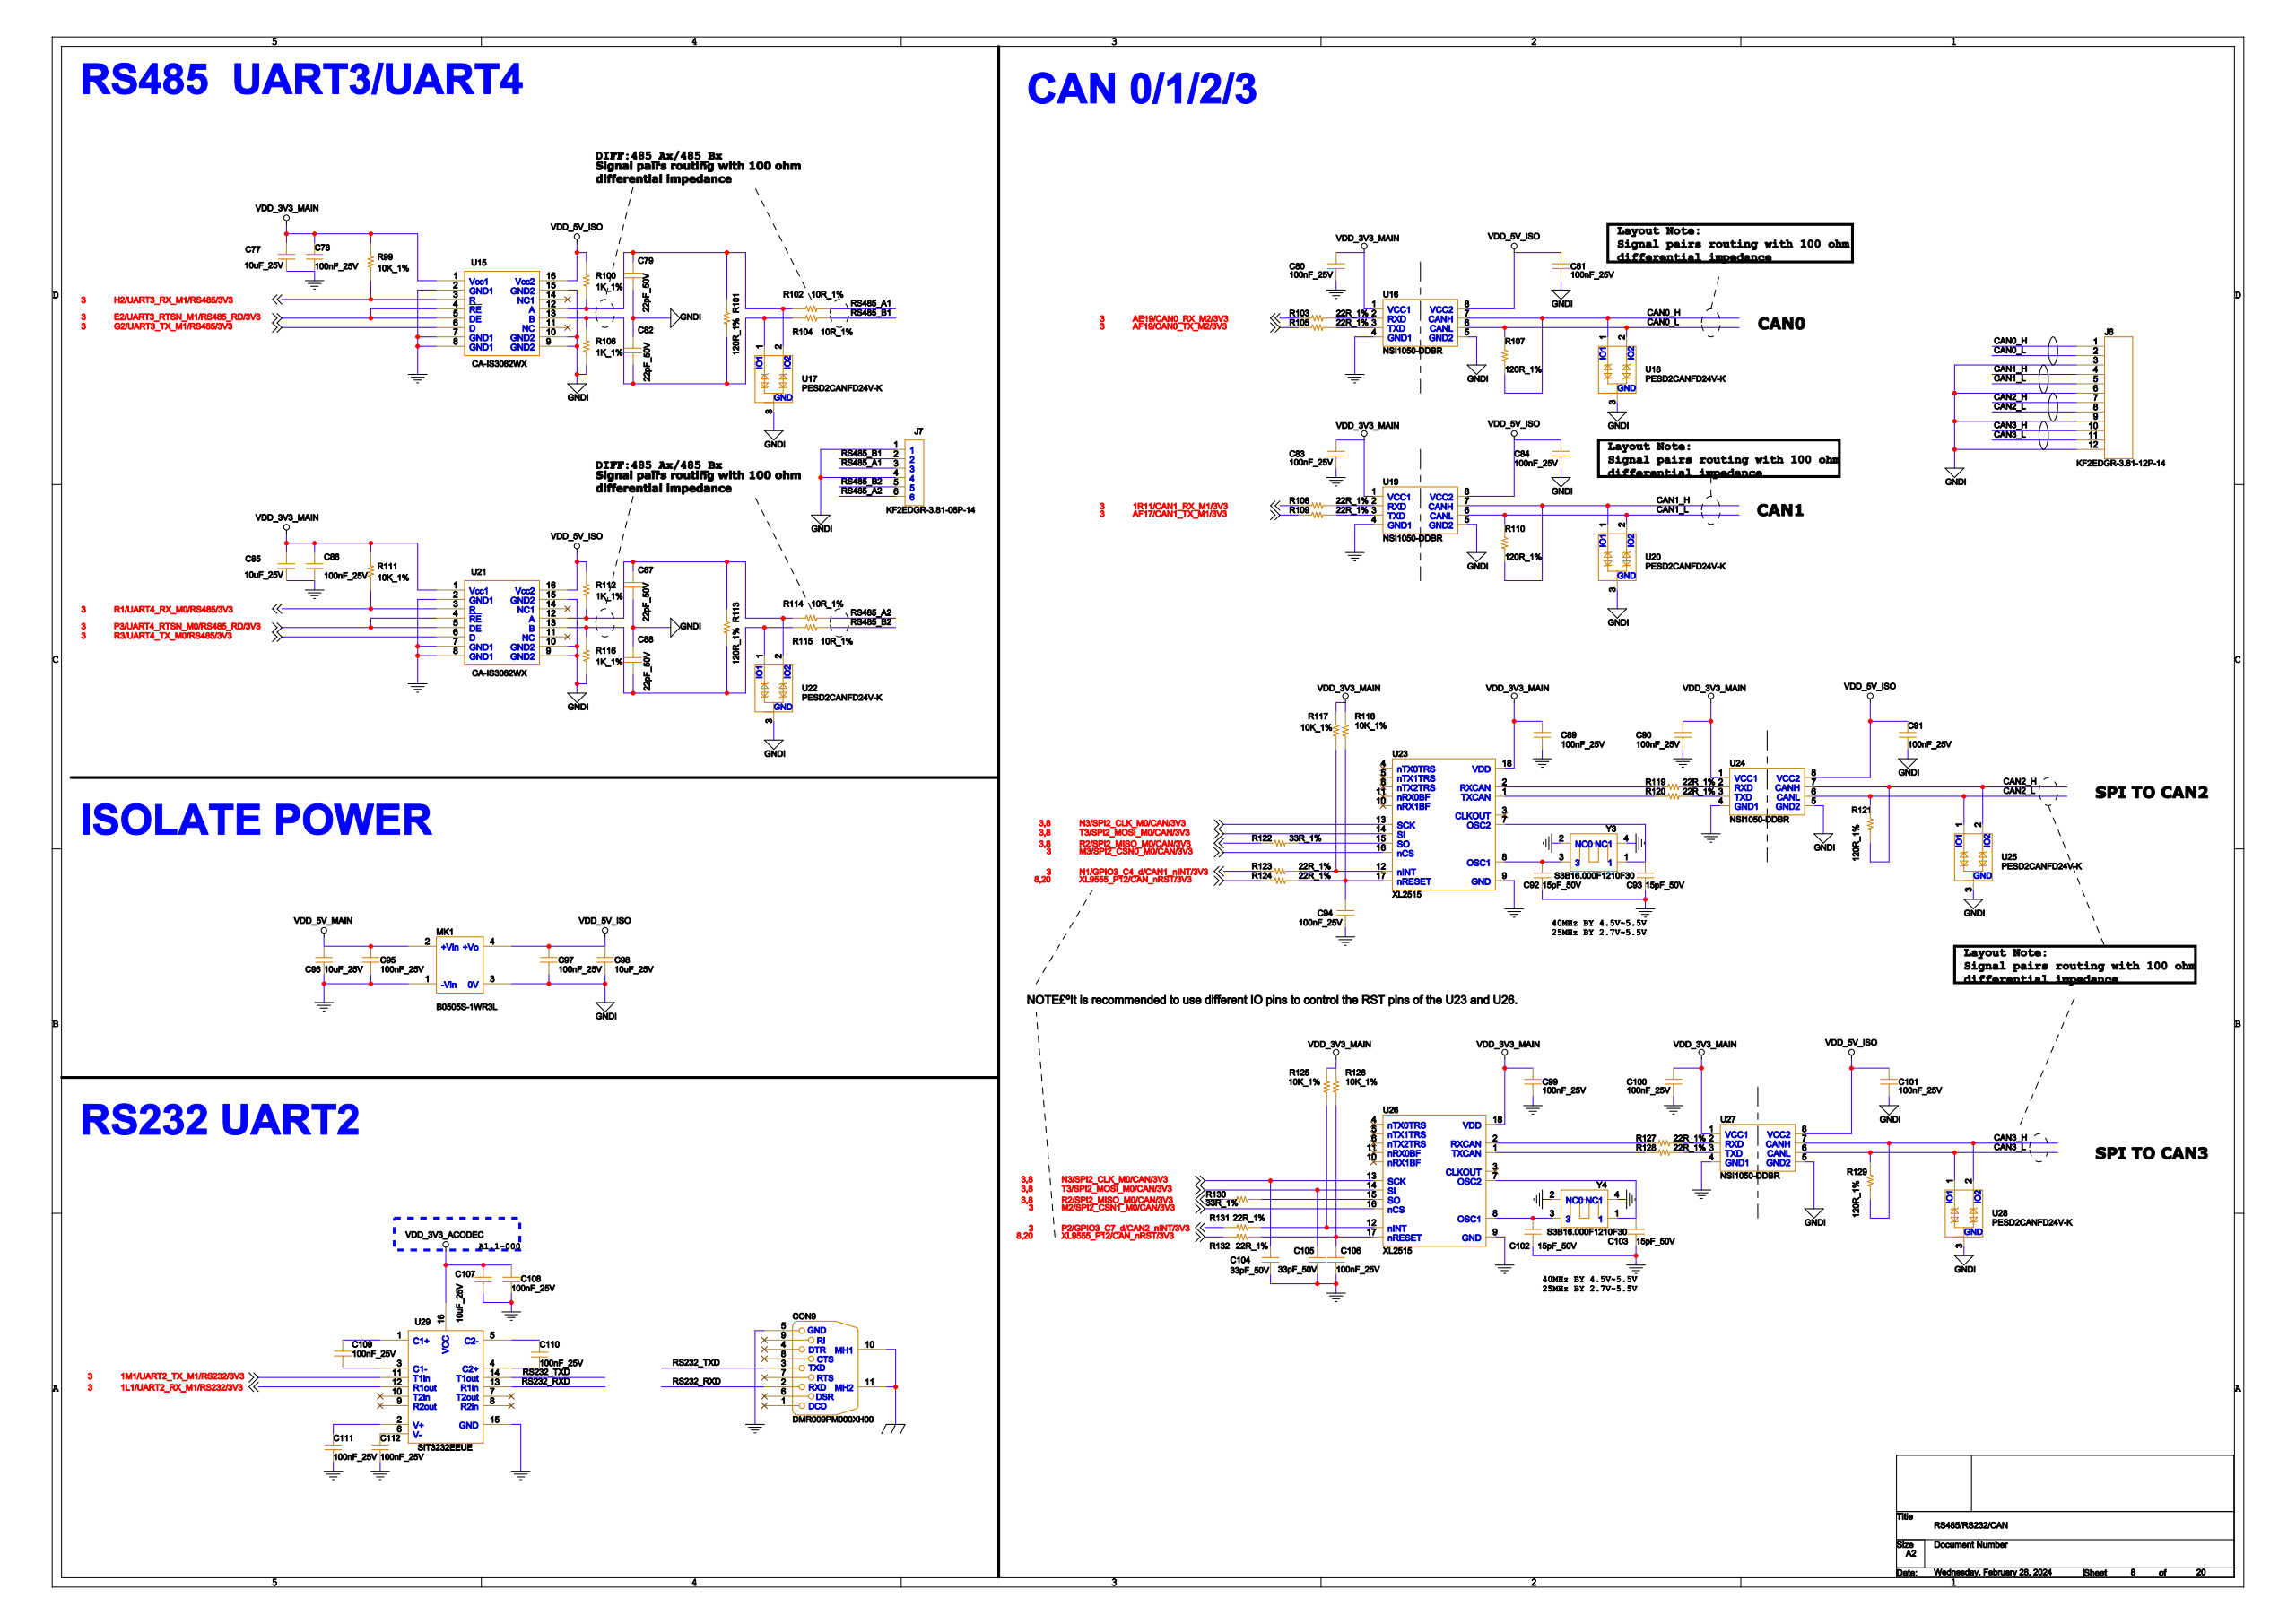Circuit board | Cadence Allegro | 1024 parts | 682 nets | one sheet of the schematic
Parts on this sheet (reference | value | footprint):
C77 | 10uF_25V | C0603
C78 | 100nF_25V | C0402
C80 | 100nF_25V | C0402
C81 | 100nF_25V | C0402
C83 | 100nF_25V | C0402
C84 | 100nF_25V | C0402
C85 | 10uF_25V | C0603
C86 | 100nF_25V | C0402
C89 | 100nF_25V | C0402
C90 | 100nF_25V | C0402
C91 | 100nF_25V | C0402
C92 | 15pF_50V | C0402
C93 | 15pF_50V | C0402
C94 | 100nF_25V | C0402
C95 | 100nF_25V | C0402
C96 | 10uF_25V | C0603
C97 | 100nF_25V | C0402
C98 | 10uF_25V | C0603
C99 | 100nF_25V | C0402
C100 | 100nF_25V | C0402
C101 | 100nF_25V | C0402
C102 | 15pF_50V | C0402
C103 | 15pF_50V | C0402
C104 | 33pF_50V | C0603
C105 | 33pF_50V | C0603
C106 | 100nF_25V | C0402
C107 | 10uF_25V | C0603
C108 | 100nF_25V | C0402
C109 | 100nF_25V | C0402
C110 | 100nF_25V | C0402
C111 | 100nF_25V | C0402
C112 | 100nF_25V | C0402
CON9 | D-DMR009PM-D002 | CON_DB9
J6 | KF2EDGR-3.81-12P | KF2EDGR-3D81-12P
J7 | KF2EDGR-3.81-06P | KF2EG_3_81-6P
MK1 | B0505S-1WR3L | DIP4_B0505S_1W
R99 | 10K_1% | R0402
R100 | 1K_1% | R0402
R101 | 120R_1% | R0805
R102 | 10R_1% | R0603
R103 | 22R_1% | R0402
R104 | 10R_1% | R0603
R105 | 22R_1% | R0402
R106 | 1K_1% | R0402
R107 | 120R_1% | R0805
R108 | 22R_1% | R0402
R109 | 22R_1% | R0402
R110 | 120R_1% | R0805
R111 | 10K_1% | R0402
R112 | 1K_1% | R0402
R113 | 120R_1% | R0805
R114 | 10R_1% | R0603
R115 | 10R_1% | R0603
R116 | 1K_1% | R0402
R117 | 10K_1% | R0402
R118 | 10K_1% | R0402
R119 | 22R_1% | R0402
R120 | 22R_1% | R0402
R121 | 120R_1% | R0805
R122 | 33R_1% | R0402
R123 | 22R_1% | R0402
R124 | 22R_1% | R0402
R125 | 10K_1% | R0402
R126 | 10K_1% | R0402
R127 | 22R_1% | R0402
R128 | 22R_1% | R0402
R129 | 120R_1% | R0805
R130 | 33R_1% | R0402
R131 | 22R_1% | R0402
R132 | 22R_1% | R0402
U15 | CA-IS3082WX | SOIC16
U16 | NSI1050-DDBR | SOP8
U17 | PESD2CANFD24V-K | SOT23-3
U18 | PESD2CANFD24V-K | SOT23-3
U19 | NSI1050-DDBR | SOP8
U20 | PESD2CANFD24V-K | SOT23-3
U21 | CA-IS3082WX | SOIC16
U22 | PESD2CANFD24V-K | SOT23-3
U23 | XL2515 | SOIC18
U24 | NSI1050-DDBR | SOP8
U25 | PESD2CANFD24V-K | SOT23-3
U26 | XL2515 | SOIC18
U27 | NSI1050-DDBR | SOP8
U28 | PESD2CANFD24V-K | SOT23-3
U29 | SIT3232EEUE | TSSOP16_PW16
Y3 | S3B16.000F1210F30 | SMD_3225
Y4 | S3B16.000F1210F30 | SMD_3225
Nets of these parts (net: part-pin ...):
GND: C77-2 C78-2 C80-2 C83-2 C85-2 C86-2 C89-2 C90-2 C92-2 C93-2 C94-2 C95-2 C96-2 C99-2 C100-2 C102-2 C103-2 C104-2 C105-2 C106-2 C107-1 C108-1 C111-2 C112-2 CON9-5 MK1-1 U15-2 U15-7 U15-8 U16-4 U19-4 U21-2 U21-7 U21-8 U23-9 U24-4 U26-9 U27-4 U29-15 Y3-2 Y3-4 Y4-2 Y4-4
VDD_5V_MAIN: C95-1 C96-1 MK1-2
VDD_3V3_ACODEC: C107-2 C108-2 U29-16
EGND: CON9-10 CON9-11
RS232_RXD: CON9-2 U29-13
RS232_TXD: CON9-3 U29-14
VDD_3V3_MAIN: C77-1 C78-1 C80-1 C83-1 C85-1 C86-1 C89-1 C90-1 C99-1 C100-1 R99-1 R111-1 R117-2 R118-2 R125-2 R126-2 U15-1 U16-1 U19-1 U21-1 U23-18 U24-1 U26-18 U27-1
N21628085: C102-1 U26-8 Y4-3
N21628083: C103-1 U26-7 Y4-1
N21627732: C92-1 U23-8 Y3-3
N21627730: C93-1 U23-7 Y3-1
AF19/CAN0_TX_M2/3V3: R105-1
AE19/CAN0_RX_M2/3V3: R103-1
AF17/CAN1_TX_M1/3V3: R109-1
1R11/CAN1_RX_M1/3V3: R108-1
1M1/UART2_TX_M1/RS232/3V3: U29-11
1L1/UART2_RX_M1/RS232/3V3: U29-12
G2/UART3_TX_M1/RS485/3V3: U15-6
H2/UART3_RX_M1/RS485/3V3: R99-2 U15-3
E2/UART3_RTSN_M1/RS485_RD/3V3: U15-4 U15-5
R1/UART4_RX_M0/RS485/3V3: R111-2 U21-3
R3/UART4_TX_M0/RS485/3V3: U21-6
N1/GPIO3_C4_D/CAN1_NINT/3V3: R123-1
P2/GPIO3_C7_D/CAN2_NINT/3V3: R131-1
P3/UART4_RTSN_M0/RS485_RD/3V3: U21-4 U21-5
M2/SPI2_CSN1_M0/CAN/3V3: U26-16
M3/SPI2_CSN0_M0/CAN/3V3: U23-16
R2/SPI2_MISO_M0/CAN/3V3: R122-1 R130-1
CAN0_H: J6-1 R107-1 U16-7 U18-1
CAN3_H: J6-10 R129-1 U27-7 U28-2
CAN3_L: J6-11 R129-2 U27-6 U28-1
GNDI: C81-2 C84-2 C91-2 C97-2 C98-2 C101-2 J6-3 J6-6 J6-9 J6-12 J7-1 J7-4 MK1-3 R106-2 R116-2 U15-9 U15-10 U15-15 U16-5 U17-3 U18-3 U19-5 U20-3 U21-9 U21-10 U21-15 U22-3 U24-5 U25-3 U27-5 U28-3
CAN0_L: J6-2 R107-2 U16-6 U18-2
CAN1_H: J6-4 R110-1 U19-7 U20-1
CAN1_L: J6-5 R110-2 U19-6 U20-2
CAN2_H: J6-7 R121-1 U24-7 U25-2
CAN2_L: J6-8 R121-2 U24-6 U25-1
RS485_B1: J7-2 R104-1
RS485_A1: J7-3 R102-1
RS485_B2: J7-5 R115-1
RS485_A2: J7-6 R114-1
VDD_5V_ISO: C81-1 C84-1 C91-1 C97-1 C98-1 C101-1 MK1-4 R100-1 R112-1 U15-16 U16-8 U19-8 U21-16 U24-8 U27-8
N21591077: R100-2 R101-1 R102-2 U15-12 U17-2
N21591075: R101-2 R104-2 R106-1 U15-13 U17-1
N21591820: R112-2 R113-1 R114-2 U21-12 U22-2
N21591818: R113-2 R115-2 R116-1 U21-13 U22-1
N21627755: R117-1 R123-2 U23-12
N21627753: C94-1 R118-1 R124-2 U23-17
N21627453: R125-1 R131-2 U26-12
N21627451: C106-1 R126-1 R132-2 U26-17
N21627545: R119-1 U23-2
N21627527: R119-2 U24-2
N21627547: R120-1 U23-1
N21627529: R120-2 U24-3
XL9555_P12/CAN_NRST/3V3: R124-1 R132-1
N21627498: R127-1 U26-2
N21628067: R127-2 U27-2
N21627496: R128-1 U26-1
N21628069: R128-2 U27-3
N21627793: R122-2 U23-15
N21627443: R130-2 U26-15
N21629181: R103-2 U16-2
N21629183: R105-2 U16-3
N21629048: R108-2 U19-2
N21628927: R109-2 U19-3
N3/SPI2_CLK_M0/CAN/3V3: C104-1 U23-13 U26-13
T3/SPI2_MOSI_M0/CAN/3V3: C105-1 U23-14 U26-14
N21592732: C110-1 U29-4
N21592722: C110-2 U29-5
N21592724: C111-1 U29-2
N21592756: C109-1 U29-1
N21592730: C109-2 U29-3
N215927860: C112-1 U29-6